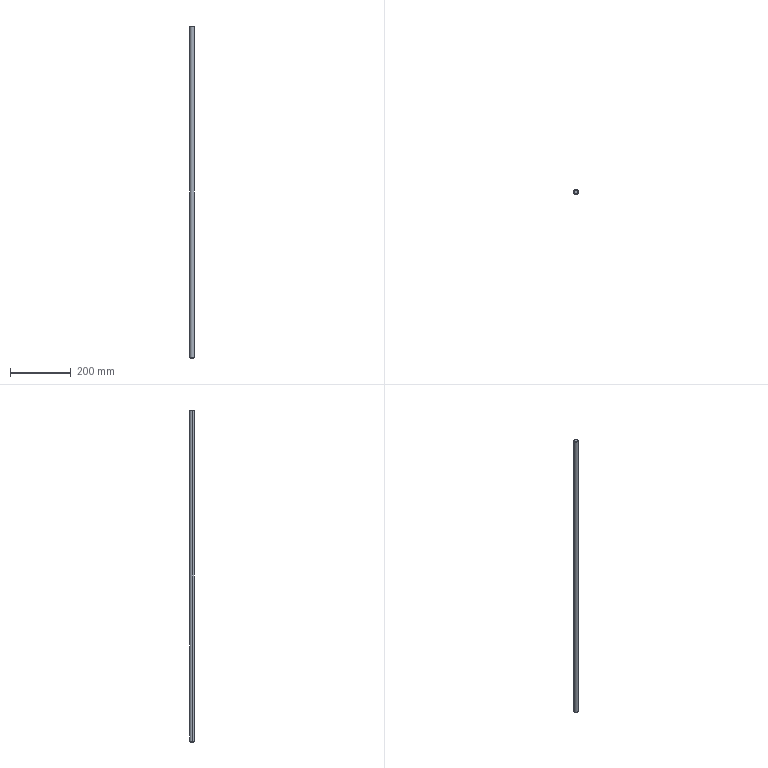Part | SolidWorks | features ICE 2, Extrusion 1, Fillet 1 | 1 solid | 13 faces | box 15 x 15 x 1090 mm | volume 192288 mm3 | torus 5 | plane 5 | cylinder 3 | commonest cylinder face diameters 15 x2 5 x1
STEP:
#1=CARTESIAN_POINT('',(-7.5,0.,543.));
#2=VERTEX_POINT('',#1);
#3=CARTESIAN_POINT('',(7.5,0.,543.));
#4=VERTEX_POINT('',#3);
#5=CARTESIAN_POINT('',(0.,0.,543.));
#6=DIRECTION('',(0.,0.,-1.));
#7=DIRECTION('',(1.,0.,0.));
#8=AXIS2_PLACEMENT_3D('',#5,#6,#7);
#9=CIRCLE('',#8,7.5);
#10=EDGE_CURVE('',#2,#4,#9,.T.);
#11=ORIENTED_EDGE('',*,*,#10,.F.);
#12=CARTESIAN_POINT('',(-5.5,0.,545.));
#13=VERTEX_POINT('',#12);
#14=CARTESIAN_POINT('',(-5.5,0.,543.));
#15=DIRECTION('',(0.,1.,0.));
#16=DIRECTION('',(-1.,0.,0.));
#17=AXIS2_PLACEMENT_3D('',#14,#15,#16);
#18=CIRCLE('',#17,2.);
#19=EDGE_CURVE('',#2,#13,#18,.T.);
#20=ORIENTED_EDGE('',*,*,#19,.T.);
#21=CARTESIAN_POINT('',(5.5,0.,545.));
#22=VERTEX_POINT('',#21);
#23=CARTESIAN_POINT('',(0.,0.,545.));
#24=DIRECTION('',(0.,0.,1.));
#25=DIRECTION('',(1.,0.,0.));
#26=AXIS2_PLACEMENT_3D('',#23,#24,#25);
#27=CIRCLE('',#26,5.5);
#28=EDGE_CURVE('',#22,#13,#27,.T.);
#29=ORIENTED_EDGE('',*,*,#28,.F.);
#30=CARTESIAN_POINT('',(5.5,0.,543.));
#31=DIRECTION('',(0.,-1.,0.));
#32=DIRECTION('',(0.,0.,-1.));
#33=AXIS2_PLACEMENT_3D('',#30,#31,#32);
#34=CIRCLE('',#33,2.);
#35=EDGE_CURVE('',#4,#22,#34,.T.);
#36=ORIENTED_EDGE('',*,*,#35,.F.);
#37=EDGE_LOOP('',(#11,#20,#29,#36));
#38=FACE_OUTER_BOUND('',#37,.T.);
#39=CARTESIAN_POINT('',(0.,0.,543.));
#40=DIRECTION('',(0.,0.,1.));
#41=DIRECTION('',(1.,0.,0.));
#42=AXIS2_PLACEMENT_3D('',#39,#40,#41);
#43=TOROIDAL_SURFACE('',#42,5.5,2.);
#44=ADVANCED_FACE('',(#38),#43,.T.);
#45=CARTESIAN_POINT('',(-5.5,0.,-545.));
#46=VERTEX_POINT('',#45);
#47=CARTESIAN_POINT('',(-2.291,5.,-545.));
#48=VERTEX_POINT('',#47);
#49=CARTESIAN_POINT('',(0.,0.,-545.));
#50=DIRECTION('',(0.,0.,-1.));
#51=DIRECTION('',(1.,0.,0.));
#52=AXIS2_PLACEMENT_3D('',#49,#50,#51);
#53=CIRCLE('',#52,5.5);
#54=EDGE_CURVE('',#46,#48,#53,.T.);
#55=ORIENTED_EDGE('',*,*,#54,.F.);
#56=CARTESIAN_POINT('',(-7.5,0.,-543.));
#57=VERTEX_POINT('',#56);
#58=CARTESIAN_POINT('',(-5.5,0.,-543.));
#59=DIRECTION('',(0.,1.,0.));
#60=DIRECTION('',(-1.,0.,0.));
#61=AXIS2_PLACEMENT_3D('',#58,#59,#60);
#62=CIRCLE('',#61,2.);
#63=EDGE_CURVE('',#46,#57,#62,.T.);
#64=ORIENTED_EDGE('',*,*,#63,.T.);
#65=CARTESIAN_POINT('',(-2.5,7.071,-543.));
#66=VERTEX_POINT('',#65);
#67=CARTESIAN_POINT('',(0.,0.,-543.));
#68=DIRECTION('',(0.,0.,1.));
#69=DIRECTION('',(1.,0.,0.));
#70=AXIS2_PLACEMENT_3D('',#67,#68,#69);
#71=CIRCLE('',#70,7.5);
#72=EDGE_CURVE('',#66,#57,#71,.T.);
#73=ORIENTED_EDGE('',*,*,#72,.F.);
#74=CARTESIAN_POINT('',(-2.5,5.,-544.998));
#75=VERTEX_POINT('',#74);
#76=CARTESIAN_POINT('',(-2.5,5.,-544.998));
#77=CARTESIAN_POINT('',(-2.5,5.264,-544.987));
#78=CARTESIAN_POINT('',(-2.5,5.53,-544.933));
#79=CARTESIAN_POINT('',(-2.5,6.021,-544.739));
#80=CARTESIAN_POINT('',(-2.5,6.252,-544.595));
#81=CARTESIAN_POINT('',(-2.5,6.542,-544.325));
#82=CARTESIAN_POINT('',(-2.5,6.631,-544.225));
#83=CARTESIAN_POINT('',(-2.5,6.786,-544.009));
#84=CARTESIAN_POINT('',(-2.5,6.852,-543.894));
#85=CARTESIAN_POINT('',(-2.5,6.96,-543.653));
#86=CARTESIAN_POINT('',(-2.5,7.002,-543.524));
#87=CARTESIAN_POINT('',(-2.5,7.057,-543.265));
#88=CARTESIAN_POINT('',(-2.5,7.071,-543.133));
#89=CARTESIAN_POINT('',(-2.5,7.071,-543.));
#90=B_SPLINE_CURVE_WITH_KNOTS('',3,(#76,#77,#78,#79,#80,#81,#82,#83,#84,#85,#86,#87,#88,#89),.UNSPECIFIED.,.F.,.F.,(4,2,2,2,2,2,4),(0.01303,0.01382,0.01461,0.01501,0.0154,0.0158,0.0162),.UNSPECIFIED.);
#91=EDGE_CURVE('',#75,#66,#90,.T.);
#92=ORIENTED_EDGE('',*,*,#91,.F.);
#93=CARTESIAN_POINT('',(-2.291,5.,-545.));
#94=CARTESIAN_POINT('',(-2.326,5.,-545.));
#95=CARTESIAN_POINT('',(-2.396,5.,-545.));
#96=CARTESIAN_POINT('',(-2.465,5.,-544.999));
#97=CARTESIAN_POINT('',(-2.5,5.,-544.998));
#98=B_SPLINE_CURVE_WITH_KNOTS('',3,(#93,#94,#95,#96,#97),.UNSPECIFIED.,.F.,.F.,(4,1,4),(0.002287,0.002392,0.002496),.UNSPECIFIED.);
#99=EDGE_CURVE('',#48,#75,#98,.T.);
#100=ORIENTED_EDGE('',*,*,#99,.F.);
#101=EDGE_LOOP('',(#55,#64,#73,#92,#100));
#102=FACE_OUTER_BOUND('',#101,.T.);
#103=CARTESIAN_POINT('',(0.,0.,-543.));
#104=DIRECTION('',(0.,0.,1.));
#105=DIRECTION('',(1.,0.,0.));
#106=AXIS2_PLACEMENT_3D('',#103,#104,#105);
#107=TOROIDAL_SURFACE('',#106,5.5,2.);
#108=ADVANCED_FACE('',(#102),#107,.T.);
#109=ORIENTED_EDGE('',*,*,#63,.F.);
#110=CARTESIAN_POINT('',(5.5,0.,-545.));
#111=VERTEX_POINT('',#110);
#112=CARTESIAN_POINT('',(0.,0.,-545.));
#113=DIRECTION('',(0.,0.,-1.));
#114=DIRECTION('',(1.,0.,0.));
#115=AXIS2_PLACEMENT_3D('',#112,#113,#114);
#116=CIRCLE('',#115,5.5);
#117=EDGE_CURVE('',#111,#46,#116,.T.);
#118=ORIENTED_EDGE('',*,*,#117,.F.);
#119=CARTESIAN_POINT('',(7.5,0.,-543.));
#120=VERTEX_POINT('',#119);
#121=CARTESIAN_POINT('',(5.5,0.,-543.));
#122=DIRECTION('',(0.,-1.,0.));
#123=DIRECTION('',(0.,0.,-1.));
#124=AXIS2_PLACEMENT_3D('',#121,#122,#123);
#125=CIRCLE('',#124,2.);
#126=EDGE_CURVE('',#111,#120,#125,.T.);
#127=ORIENTED_EDGE('',*,*,#126,.T.);
#128=CARTESIAN_POINT('',(0.,0.,-543.));
#129=DIRECTION('',(0.,0.,1.));
#130=DIRECTION('',(1.,0.,0.));
#131=AXIS2_PLACEMENT_3D('',#128,#129,#130);
#132=CIRCLE('',#131,7.5);
#133=EDGE_CURVE('',#57,#120,#132,.T.);
#134=ORIENTED_EDGE('',*,*,#133,.F.);
#135=EDGE_LOOP('',(#109,#118,#127,#134));
#136=FACE_OUTER_BOUND('',#135,.T.);
#137=CARTESIAN_POINT('',(0.,0.,-543.));
#138=DIRECTION('',(0.,0.,1.));
#139=DIRECTION('',(1.,0.,0.));
#140=AXIS2_PLACEMENT_3D('',#137,#138,#139);
#141=TOROIDAL_SURFACE('',#140,5.5,2.);
#142=ADVANCED_FACE('',(#136),#141,.T.);
#143=ORIENTED_EDGE('',*,*,#10,.T.);
#144=CARTESIAN_POINT('',(7.5,0.,545.));
#145=DIRECTION('',(0.,0.,-1.));
#146=VECTOR('',#145,1000.);
#147=LINE('',#144,#146);
#148=EDGE_CURVE('',#4,#120,#147,.T.);
#149=ORIENTED_EDGE('',*,*,#148,.T.);
#150=CARTESIAN_POINT('',(2.5,7.071,-543.));
#151=VERTEX_POINT('',#150);
#152=CARTESIAN_POINT('',(0.,0.,-543.));
#153=DIRECTION('',(0.,0.,1.));
#154=DIRECTION('',(1.,0.,0.));
#155=AXIS2_PLACEMENT_3D('',#152,#153,#154);
#156=CIRCLE('',#155,7.5);
#157=EDGE_CURVE('',#120,#151,#156,.T.);
#158=ORIENTED_EDGE('',*,*,#157,.T.);
#159=CARTESIAN_POINT('',(2.5,7.071,-525.));
#160=VERTEX_POINT('',#159);
#161=CARTESIAN_POINT('',(2.5,7.071,545.));
#162=DIRECTION('',(0.,0.,1.));
#163=VECTOR('',#162,1000.);
#164=LINE('',#161,#163);
#165=EDGE_CURVE('',#151,#160,#164,.T.);
#166=ORIENTED_EDGE('',*,*,#165,.T.);
#167=CARTESIAN_POINT('',(-2.5,7.071,-525.));
#168=VERTEX_POINT('',#167);
#169=CARTESIAN_POINT('',(-2.5,7.071,-525.));
#170=CARTESIAN_POINT('',(-2.5,7.071,-524.836));
#171=CARTESIAN_POINT('',(-2.483,7.077,-524.669));
#172=CARTESIAN_POINT('',(-2.419,7.099,-524.347));
#173=CARTESIAN_POINT('',(-2.371,7.116,-524.191));
#174=CARTESIAN_POINT('',(-2.244,7.157,-523.887));
#175=CARTESIAN_POINT('',(-2.167,7.181,-523.743));
#176=CARTESIAN_POINT('',(-1.986,7.233,-523.473));
#177=CARTESIAN_POINT('',(-1.882,7.261,-523.346));
#178=CARTESIAN_POINT('',(-1.652,7.317,-523.116));
#179=CARTESIAN_POINT('',(-1.527,7.344,-523.014));
#180=CARTESIAN_POINT('',(-1.257,7.395,-522.833));
#181=CARTESIAN_POINT('',(-1.11,7.419,-522.754));
#182=CARTESIAN_POINT('',(-0.8093,7.458,-522.629));
#183=CARTESIAN_POINT('',(-0.6533,7.473,-522.581));
#184=CARTESIAN_POINT('',(-0.3296,7.495,-522.516));
#185=CARTESIAN_POINT('',(-0.164,7.5,-522.5));
#186=CARTESIAN_POINT('',(0.1639,7.5,-522.5));
#187=CARTESIAN_POINT('',(0.329,7.495,-522.516));
#188=CARTESIAN_POINT('',(0.6533,7.473,-522.581));
#189=CARTESIAN_POINT('',(0.8096,7.458,-522.629));
#190=CARTESIAN_POINT('',(1.111,7.419,-522.755));
#191=CARTESIAN_POINT('',(1.257,7.395,-522.833));
#192=CARTESIAN_POINT('',(1.527,7.344,-523.014));
#193=CARTESIAN_POINT('',(1.653,7.317,-523.117));
#194=CARTESIAN_POINT('',(1.999,7.233,-523.463));
#195=CARTESIAN_POINT('',(2.182,7.177,-523.736));
#196=CARTESIAN_POINT('',(2.371,7.116,-524.192));
#197=CARTESIAN_POINT('',(2.419,7.099,-524.348));
#198=CARTESIAN_POINT('',(2.483,7.077,-524.669));
#199=CARTESIAN_POINT('',(2.5,7.071,-524.835));
#200=CARTESIAN_POINT('',(2.5,7.071,-525.));
#201=B_SPLINE_CURVE_WITH_KNOTS('',3,(#169,#170,#171,#172,#173,#174,#175,#176,#177,#178,#179,#180,#181,#182,#183,#184,#185,#186,#187,#188,#189,#190,#191,#192,#193,#194,#195,#196,#197,#198,#199,#200),.UNSPECIFIED.,.F.,.F.,(4,2,2,2,2,2,2,2,2,2,2,2,2,2,2,4),(0.003938,0.00443,0.004921,0.005413,0.005905,0.006397,0.006889,0.007381,0.007873,0.008365,0.008857,0.009349,0.00984,0.01082,0.01132,0.01181),.UNSPECIFIED.);
#202=EDGE_CURVE('',#168,#160,#201,.T.);
#203=ORIENTED_EDGE('',*,*,#202,.F.);
#204=CARTESIAN_POINT('',(-2.5,7.071,545.));
#205=DIRECTION('',(0.,0.,-1.));
#206=VECTOR('',#205,1000.);
#207=LINE('',#204,#206);
#208=EDGE_CURVE('',#168,#66,#207,.T.);
#209=ORIENTED_EDGE('',*,*,#208,.T.);
#210=ORIENTED_EDGE('',*,*,#72,.T.);
#211=CARTESIAN_POINT('',(-7.5,0.,545.));
#212=DIRECTION('',(0.,0.,-1.));
#213=VECTOR('',#212,1000.);
#214=LINE('',#211,#213);
#215=EDGE_CURVE('',#2,#57,#214,.T.);
#216=ORIENTED_EDGE('',*,*,#215,.F.);
#217=EDGE_LOOP('',(#143,#149,#158,#166,#203,#209,#210,#216));
#218=FACE_OUTER_BOUND('',#217,.T.);
#219=CARTESIAN_POINT('',(0.,0.,545.));
#220=DIRECTION('',(0.,0.,-1.));
#221=DIRECTION('',(-1.,0.,0.));
#222=AXIS2_PLACEMENT_3D('',#219,#220,#221);
#223=CYLINDRICAL_SURFACE('',#222,7.5);
#224=ADVANCED_FACE('',(#218),#223,.T.);
#225=ORIENTED_EDGE('',*,*,#148,.F.);
#226=CARTESIAN_POINT('',(0.,0.,543.));
#227=DIRECTION('',(0.,0.,-1.));
#228=DIRECTION('',(1.,0.,0.));
#229=AXIS2_PLACEMENT_3D('',#226,#227,#228);
#230=CIRCLE('',#229,7.5);
#231=EDGE_CURVE('',#4,#2,#230,.T.);
#232=ORIENTED_EDGE('',*,*,#231,.T.);
#233=ORIENTED_EDGE('',*,*,#215,.T.);
#234=ORIENTED_EDGE('',*,*,#133,.T.);
#235=EDGE_LOOP('',(#225,#232,#233,#234));
#236=FACE_OUTER_BOUND('',#235,.T.);
#237=CARTESIAN_POINT('',(0.,0.,545.));
#238=DIRECTION('',(0.,0.,-1.));
#239=DIRECTION('',(-1.,0.,0.));
#240=AXIS2_PLACEMENT_3D('',#237,#238,#239);
#241=CYLINDRICAL_SURFACE('',#240,7.5);
#242=ADVANCED_FACE('',(#236),#241,.T.);
#243=ORIENTED_EDGE('',*,*,#28,.T.);
#244=CARTESIAN_POINT('',(0.,0.,545.));
#245=DIRECTION('',(0.,0.,1.));
#246=DIRECTION('',(1.,0.,0.));
#247=AXIS2_PLACEMENT_3D('',#244,#245,#246);
#248=CIRCLE('',#247,5.5);
#249=EDGE_CURVE('',#13,#22,#248,.T.);
#250=ORIENTED_EDGE('',*,*,#249,.T.);
#251=EDGE_LOOP('',(#243,#250));
#252=FACE_OUTER_BOUND('',#251,.T.);
#253=CARTESIAN_POINT('',(0.,0.,545.));
#254=DIRECTION('',(0.,0.,1.));
#255=DIRECTION('',(1.,0.,0.));
#256=AXIS2_PLACEMENT_3D('',#253,#254,#255);
#257=PLANE('',#256);
#258=ADVANCED_FACE('',(#252),#257,.T.);
#259=CARTESIAN_POINT('',(2.291,5.,-545.));
#260=VERTEX_POINT('',#259);
#261=CARTESIAN_POINT('',(0.,0.,-545.));
#262=DIRECTION('',(0.,0.,-1.));
#263=DIRECTION('',(1.,0.,0.));
#264=AXIS2_PLACEMENT_3D('',#261,#262,#263);
#265=CIRCLE('',#264,5.5);
#266=EDGE_CURVE('',#260,#111,#265,.T.);
#267=ORIENTED_EDGE('',*,*,#266,.T.);
#268=ORIENTED_EDGE('',*,*,#117,.T.);
#269=ORIENTED_EDGE('',*,*,#54,.T.);
#270=CARTESIAN_POINT('',(2.5,5.,-545.));
#271=DIRECTION('',(-1.,0.,0.));
#272=VECTOR('',#271,1000.);
#273=LINE('',#270,#272);
#274=EDGE_CURVE('',#260,#48,#273,.T.);
#275=ORIENTED_EDGE('',*,*,#274,.F.);
#276=EDGE_LOOP('',(#267,#268,#269,#275));
#277=FACE_OUTER_BOUND('',#276,.T.);
#278=CARTESIAN_POINT('',(0.,0.,-545.));
#279=DIRECTION('',(0.,0.,1.));
#280=DIRECTION('',(1.,0.,0.));
#281=AXIS2_PLACEMENT_3D('',#278,#279,#280);
#282=PLANE('',#281);
#283=ADVANCED_FACE('',(#277),#282,.F.);
#284=ORIENTED_EDGE('',*,*,#126,.F.);
#285=ORIENTED_EDGE('',*,*,#266,.F.);
#286=CARTESIAN_POINT('',(2.5,5.,-544.998));
#287=VERTEX_POINT('',#286);
#288=CARTESIAN_POINT('',(2.5,5.,-544.998));
#289=CARTESIAN_POINT('',(2.465,5.,-544.999));
#290=CARTESIAN_POINT('',(2.396,5.,-545.));
#291=CARTESIAN_POINT('',(2.326,5.,-545.));
#292=CARTESIAN_POINT('',(2.291,5.,-545.));
#293=B_SPLINE_CURVE_WITH_KNOTS('',3,(#288,#289,#290,#291,#292),.UNSPECIFIED.,.F.,.F.,(4,1,4),(0.02322,0.02333,0.02343),.UNSPECIFIED.);
#294=EDGE_CURVE('',#287,#260,#293,.T.);
#295=ORIENTED_EDGE('',*,*,#294,.F.);
#296=CARTESIAN_POINT('',(2.5,7.071,-543.));
#297=CARTESIAN_POINT('',(2.5,7.071,-543.264));
#298=CARTESIAN_POINT('',(2.5,7.014,-543.53));
#299=CARTESIAN_POINT('',(2.5,6.853,-543.893));
#300=CARTESIAN_POINT('',(2.5,6.785,-544.01));
#301=CARTESIAN_POINT('',(2.5,6.631,-544.225));
#302=CARTESIAN_POINT('',(2.5,6.543,-544.324));
#303=CARTESIAN_POINT('',(2.5,6.251,-544.596));
#304=CARTESIAN_POINT('',(2.5,6.023,-544.738));
#305=CARTESIAN_POINT('',(2.5,5.527,-544.934));
#306=CARTESIAN_POINT('',(2.5,5.263,-544.987));
#307=CARTESIAN_POINT('',(2.5,5.,-544.998));
#308=B_SPLINE_CURVE_WITH_KNOTS('',3,(#296,#297,#298,#299,#300,#301,#302,#303,#304,#305,#306,#307),.UNSPECIFIED.,.F.,.F.,(4,2,2,2,2,4),(0.01068,0.01147,0.01186,0.01226,0.01305,0.01384),.UNSPECIFIED.);
#309=EDGE_CURVE('',#151,#287,#308,.T.);
#310=ORIENTED_EDGE('',*,*,#309,.F.);
#311=ORIENTED_EDGE('',*,*,#157,.F.);
#312=EDGE_LOOP('',(#284,#285,#295,#310,#311));
#313=FACE_OUTER_BOUND('',#312,.T.);
#314=CARTESIAN_POINT('',(0.,0.,-543.));
#315=DIRECTION('',(0.,0.,1.));
#316=DIRECTION('',(1.,0.,0.));
#317=AXIS2_PLACEMENT_3D('',#314,#315,#316);
#318=TOROIDAL_SURFACE('',#317,5.5,2.);
#319=ADVANCED_FACE('',(#313),#318,.T.);
#320=ORIENTED_EDGE('',*,*,#19,.F.);
#321=ORIENTED_EDGE('',*,*,#231,.F.);
#322=ORIENTED_EDGE('',*,*,#35,.T.);
#323=ORIENTED_EDGE('',*,*,#249,.F.);
#324=EDGE_LOOP('',(#320,#321,#322,#323));
#325=FACE_OUTER_BOUND('',#324,.T.);
#326=CARTESIAN_POINT('',(0.,0.,543.));
#327=DIRECTION('',(0.,0.,1.));
#328=DIRECTION('',(1.,0.,0.));
#329=AXIS2_PLACEMENT_3D('',#326,#327,#328);
#330=TOROIDAL_SURFACE('',#329,5.5,2.);
#331=ADVANCED_FACE('',(#325),#330,.T.);
#332=ORIENTED_EDGE('',*,*,#309,.T.);
#333=CARTESIAN_POINT('',(2.5,5.,-525.));
#334=VERTEX_POINT('',#333);
#335=CARTESIAN_POINT('',(2.5,5.,-525.));
#336=DIRECTION('',(0.,0.,-1.));
#337=VECTOR('',#336,1000.);
#338=LINE('',#335,#337);
#339=EDGE_CURVE('',#334,#287,#338,.T.);
#340=ORIENTED_EDGE('',*,*,#339,.F.);
#341=CARTESIAN_POINT('',(2.5,5.,-525.));
#342=DIRECTION('',(0.,-1.,0.));
#343=VECTOR('',#342,1000.);
#344=LINE('',#341,#343);
#345=EDGE_CURVE('',#160,#334,#344,.T.);
#346=ORIENTED_EDGE('',*,*,#345,.F.);
#347=ORIENTED_EDGE('',*,*,#165,.F.);
#348=EDGE_LOOP('',(#332,#340,#346,#347));
#349=FACE_OUTER_BOUND('',#348,.T.);
#350=CARTESIAN_POINT('',(2.5,5.,-525.));
#351=DIRECTION('',(1.,0.,0.));
#352=DIRECTION('',(0.,0.,-1.));
#353=AXIS2_PLACEMENT_3D('',#350,#351,#352);
#354=PLANE('',#353);
#355=ADVANCED_FACE('',(#349),#354,.F.);
#356=CARTESIAN_POINT('',(-2.5,5.,-525.));
#357=VERTEX_POINT('',#356);
#358=CARTESIAN_POINT('',(-2.5,11.77,-525.));
#359=DIRECTION('',(0.,1.,0.));
#360=VECTOR('',#359,1000.);
#361=LINE('',#358,#360);
#362=EDGE_CURVE('',#357,#168,#361,.T.);
#363=ORIENTED_EDGE('',*,*,#362,.F.);
#364=CARTESIAN_POINT('',(-2.5,5.,-525.));
#365=DIRECTION('',(0.,0.,-1.));
#366=VECTOR('',#365,1000.);
#367=LINE('',#364,#366);
#368=EDGE_CURVE('',#357,#75,#367,.T.);
#369=ORIENTED_EDGE('',*,*,#368,.T.);
#370=ORIENTED_EDGE('',*,*,#91,.T.);
#371=ORIENTED_EDGE('',*,*,#208,.F.);
#372=EDGE_LOOP('',(#363,#369,#370,#371));
#373=FACE_OUTER_BOUND('',#372,.T.);
#374=CARTESIAN_POINT('',(-2.5,11.77,-525.));
#375=DIRECTION('',(-1.,0.,0.));
#376=DIRECTION('',(0.,-1.,0.));
#377=AXIS2_PLACEMENT_3D('',#374,#375,#376);
#378=PLANE('',#377);
#379=ADVANCED_FACE('',(#373),#378,.F.);
#380=ORIENTED_EDGE('',*,*,#368,.F.);
#381=CARTESIAN_POINT('',(0.,5.,-525.));
#382=DIRECTION('',(0.,1.,0.));
#383=DIRECTION('',(0.,0.,1.));
#384=AXIS2_PLACEMENT_3D('',#381,#382,#383);
#385=CIRCLE('',#384,2.5);
#386=EDGE_CURVE('',#357,#334,#385,.T.);
#387=ORIENTED_EDGE('',*,*,#386,.T.);
#388=ORIENTED_EDGE('',*,*,#339,.T.);
#389=ORIENTED_EDGE('',*,*,#294,.T.);
#390=ORIENTED_EDGE('',*,*,#274,.T.);
#391=ORIENTED_EDGE('',*,*,#99,.T.);
#392=EDGE_LOOP('',(#380,#387,#388,#389,#390,#391));
#393=FACE_OUTER_BOUND('',#392,.T.);
#394=CARTESIAN_POINT('',(2.5,5.,-525.));
#395=DIRECTION('',(0.,-1.,0.));
#396=DIRECTION('',(0.,0.,-1.));
#397=AXIS2_PLACEMENT_3D('',#394,#395,#396);
#398=PLANE('',#397);
#399=ADVANCED_FACE('',(#393),#398,.F.);
#400=ORIENTED_EDGE('',*,*,#386,.F.);
#401=ORIENTED_EDGE('',*,*,#362,.T.);
#402=ORIENTED_EDGE('',*,*,#202,.T.);
#403=ORIENTED_EDGE('',*,*,#345,.T.);
#404=EDGE_LOOP('',(#400,#401,#402,#403));
#405=FACE_OUTER_BOUND('',#404,.T.);
#406=CARTESIAN_POINT('',(0.,7.5,-525.));
#407=DIRECTION('',(0.,-1.,0.));
#408=DIRECTION('',(0.,0.,-1.));
#409=AXIS2_PLACEMENT_3D('',#406,#407,#408);
#410=CYLINDRICAL_SURFACE('',#409,2.5);
#411=ADVANCED_FACE('',(#405),#410,.F.);
#412=CLOSED_SHELL('',(#44,#108,#142,#224,#242,#258,#283,#319,#331,#355,#379,#399,#411));
#413=MANIFOLD_SOLID_BREP('',#412);
#414=CARTESIAN_POINT('',(0.,0.,0.));
#415=DIRECTION('',(0.,0.,1.));
#416=DIRECTION('',(1.,0.,0.));
#417=AXIS2_PLACEMENT_3D('',#414,#415,#416);
#418=(LENGTH_UNIT()NAMED_UNIT(*)SI_UNIT(.MILLI.,.METRE.));
#419=UNCERTAINTY_MEASURE_WITH_UNIT(LENGTH_MEASURE(0.00001),#418,'','');
#420=(NAMED_UNIT(*)PLANE_ANGLE_UNIT()SI_UNIT($,.RADIAN.));
#421=(NAMED_UNIT(*)SI_UNIT($,.STERADIAN.)SOLID_ANGLE_UNIT());
#422=(GEOMETRIC_REPRESENTATION_CONTEXT(3)GLOBAL_UNCERTAINTY_ASSIGNED_CONTEXT((#419))GLOBAL_UNIT_ASSIGNED_CONTEXT((#418,#420,#421))REPRESENTATION_CONTEXT('',''));
#423=ADVANCED_BREP_SHAPE_REPRESENTATION('',(#413,#417),#422);